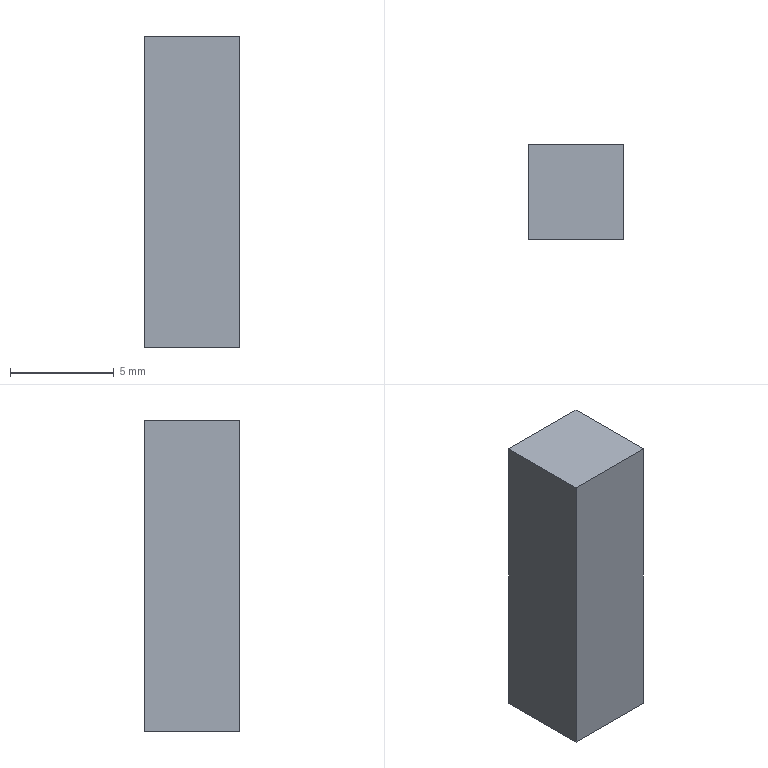Part | STEP file | Harpoon track spring pin | 1 solid | 6 faces | box 4.58 x 4.58 x 15 mm | volume 314.646 mm3 | plane 6
STEP:
#1=CARTESIAN_POINT('',(0.,0.,0.));
#2=DIRECTION('',(0.,0.,1.));
#3=DIRECTION('',(1.,0.,0.));
#4=AXIS2_PLACEMENT_3D('',#1,#2,#3);
#5=CARTESIAN_POINT('',(0.,4.58,0.));
#6=VERTEX_POINT('',#5);
#7=CARTESIAN_POINT('',(0.,0.,0.));
#8=VERTEX_POINT('',#7);
#9=CARTESIAN_POINT('',(0.,0.,0.));
#10=DIRECTION('',(0.,-1.,0.));
#11=VECTOR('',#10,1.);
#12=LINE('',#9,#11);
#13=CARTESIAN_POINT('',(0.,0.,15.));
#14=DIRECTION('',(1.,0.,0.));
#15=DIRECTION('',(0.,1.,0.));
#16=AXIS2_PLACEMENT_3D('',#13,#14,#15);
#17=PLANE('',#16);
#18=CARTESIAN_POINT('',(0.,-15.));
#19=DIRECTION('',(-1.,0.));
#20=VECTOR('',#19,1.);
#21=LINE('',#18,#20);
#22=(GEOMETRIC_REPRESENTATION_CONTEXT(2)PARAMETRIC_REPRESENTATION_CONTEXT()REPRESENTATION_CONTEXT('',''));
#23=DEFINITIONAL_REPRESENTATION('',(#21),#22);
#24=PCURVE('',#17,#23);
#25=CARTESIAN_POINT('',(0.,4.58,0.));
#26=DIRECTION('',(0.,0.,-1.));
#27=DIRECTION('',(-1.,0.,0.));
#28=AXIS2_PLACEMENT_3D('',#25,#26,#27);
#29=PLANE('',#28);
#30=CARTESIAN_POINT('',(0.,-4.58));
#31=DIRECTION('',(0.,-1.));
#32=VECTOR('',#31,1.);
#33=LINE('',#30,#32);
#34=(GEOMETRIC_REPRESENTATION_CONTEXT(2)PARAMETRIC_REPRESENTATION_CONTEXT()REPRESENTATION_CONTEXT('',''));
#35=DEFINITIONAL_REPRESENTATION('',(#33),#34);
#36=PCURVE('',#29,#35);
#37=SURFACE_CURVE('',#12,(#24,#36),.PCURVE_S1.);
#38=EDGE_CURVE('',#6,#8,#37,.T.);
#39=ORIENTED_EDGE('',*,*,#38,.T.);
#40=CARTESIAN_POINT('',(0.,0.,15.));
#41=VERTEX_POINT('',#40);
#42=CARTESIAN_POINT('',(0.,0.,15.));
#43=DIRECTION('',(0.,0.,-1.));
#44=VECTOR('',#43,1.);
#45=LINE('',#42,#44);
#46=CARTESIAN_POINT('',(0.,0.));
#47=DIRECTION('',(0.,-1.));
#48=VECTOR('',#47,1.);
#49=LINE('',#46,#48);
#50=(GEOMETRIC_REPRESENTATION_CONTEXT(2)PARAMETRIC_REPRESENTATION_CONTEXT()REPRESENTATION_CONTEXT('',''));
#51=DEFINITIONAL_REPRESENTATION('',(#49),#50);
#52=PCURVE('',#17,#51);
#53=CARTESIAN_POINT('',(0.,0.,15.));
#54=DIRECTION('',(0.,1.,0.));
#55=DIRECTION('',(0.,0.,1.));
#56=AXIS2_PLACEMENT_3D('',#53,#54,#55);
#57=PLANE('',#56);
#58=CARTESIAN_POINT('',(0.,0.));
#59=DIRECTION('',(-1.,0.));
#60=VECTOR('',#59,1.);
#61=LINE('',#58,#60);
#62=(GEOMETRIC_REPRESENTATION_CONTEXT(2)PARAMETRIC_REPRESENTATION_CONTEXT()REPRESENTATION_CONTEXT('',''));
#63=DEFINITIONAL_REPRESENTATION('',(#61),#62);
#64=PCURVE('',#57,#63);
#65=SURFACE_CURVE('',#45,(#52,#64),.PCURVE_S1.);
#66=EDGE_CURVE('',#41,#8,#65,.T.);
#67=ORIENTED_EDGE('',*,*,#66,.F.);
#68=CARTESIAN_POINT('',(0.,4.58,15.));
#69=VERTEX_POINT('',#68);
#70=CARTESIAN_POINT('',(0.,0.,15.));
#71=DIRECTION('',(0.,-1.,0.));
#72=VECTOR('',#71,1.);
#73=LINE('',#70,#72);
#74=CARTESIAN_POINT('',(0.,0.));
#75=DIRECTION('',(-1.,0.));
#76=VECTOR('',#75,1.);
#77=LINE('',#74,#76);
#78=(GEOMETRIC_REPRESENTATION_CONTEXT(2)PARAMETRIC_REPRESENTATION_CONTEXT()REPRESENTATION_CONTEXT('',''));
#79=DEFINITIONAL_REPRESENTATION('',(#77),#78);
#80=PCURVE('',#17,#79);
#81=CARTESIAN_POINT('',(0.,4.58,15.));
#82=DIRECTION('',(0.,0.,-1.));
#83=DIRECTION('',(-1.,0.,0.));
#84=AXIS2_PLACEMENT_3D('',#81,#82,#83);
#85=PLANE('',#84);
#86=CARTESIAN_POINT('',(0.,-4.58));
#87=DIRECTION('',(0.,-1.));
#88=VECTOR('',#87,1.);
#89=LINE('',#86,#88);
#90=(GEOMETRIC_REPRESENTATION_CONTEXT(2)PARAMETRIC_REPRESENTATION_CONTEXT()REPRESENTATION_CONTEXT('',''));
#91=DEFINITIONAL_REPRESENTATION('',(#89),#90);
#92=PCURVE('',#85,#91);
#93=SURFACE_CURVE('',#73,(#80,#92),.PCURVE_S1.);
#94=EDGE_CURVE('',#69,#41,#93,.T.);
#95=ORIENTED_EDGE('',*,*,#94,.F.);
#96=CARTESIAN_POINT('',(0.,4.58,15.));
#97=DIRECTION('',(0.,0.,-1.));
#98=VECTOR('',#97,1.);
#99=LINE('',#96,#98);
#100=CARTESIAN_POINT('',(4.58,0.));
#101=DIRECTION('',(0.,-1.));
#102=VECTOR('',#101,1.);
#103=LINE('',#100,#102);
#104=(GEOMETRIC_REPRESENTATION_CONTEXT(2)PARAMETRIC_REPRESENTATION_CONTEXT()REPRESENTATION_CONTEXT('',''));
#105=DEFINITIONAL_REPRESENTATION('',(#103),#104);
#106=PCURVE('',#17,#105);
#107=CARTESIAN_POINT('',(0.,4.58,15.));
#108=DIRECTION('',(0.,-1.,0.));
#109=DIRECTION('',(0.,0.,-1.));
#110=AXIS2_PLACEMENT_3D('',#107,#108,#109);
#111=PLANE('',#110);
#112=CARTESIAN_POINT('',(0.,0.));
#113=DIRECTION('',(1.,0.));
#114=VECTOR('',#113,1.);
#115=LINE('',#112,#114);
#116=(GEOMETRIC_REPRESENTATION_CONTEXT(2)PARAMETRIC_REPRESENTATION_CONTEXT()REPRESENTATION_CONTEXT('',''));
#117=DEFINITIONAL_REPRESENTATION('',(#115),#116);
#118=PCURVE('',#111,#117);
#119=SURFACE_CURVE('',#99,(#106,#118),.PCURVE_S1.);
#120=EDGE_CURVE('',#69,#6,#119,.T.);
#121=ORIENTED_EDGE('',*,*,#120,.T.);
#122=EDGE_LOOP('',(#39,#67,#95,#121));
#123=FACE_BOUND('',#122,.T.);
#124=ADVANCED_FACE('',(#123),#17,.F.);
#125=CARTESIAN_POINT('',(4.58,0.,0.));
#126=VERTEX_POINT('',#125);
#127=CARTESIAN_POINT('',(0.,0.,0.));
#128=DIRECTION('',(1.,0.,0.));
#129=VECTOR('',#128,1.);
#130=LINE('',#127,#129);
#131=CARTESIAN_POINT('',(-15.,0.));
#132=DIRECTION('',(0.,1.));
#133=VECTOR('',#132,1.);
#134=LINE('',#131,#133);
#135=(GEOMETRIC_REPRESENTATION_CONTEXT(2)PARAMETRIC_REPRESENTATION_CONTEXT()REPRESENTATION_CONTEXT('',''));
#136=DEFINITIONAL_REPRESENTATION('',(#134),#135);
#137=PCURVE('',#57,#136);
#138=CARTESIAN_POINT('',(0.,-4.58));
#139=DIRECTION('',(-1.,0.));
#140=VECTOR('',#139,1.);
#141=LINE('',#138,#140);
#142=(GEOMETRIC_REPRESENTATION_CONTEXT(2)PARAMETRIC_REPRESENTATION_CONTEXT()REPRESENTATION_CONTEXT('',''));
#143=DEFINITIONAL_REPRESENTATION('',(#141),#142);
#144=PCURVE('',#29,#143);
#145=SURFACE_CURVE('',#130,(#137,#144),.PCURVE_S1.);
#146=EDGE_CURVE('',#8,#126,#145,.T.);
#147=ORIENTED_EDGE('',*,*,#146,.T.);
#148=CARTESIAN_POINT('',(4.58,0.,15.));
#149=VERTEX_POINT('',#148);
#150=CARTESIAN_POINT('',(4.58,0.,15.));
#151=DIRECTION('',(0.,0.,-1.));
#152=VECTOR('',#151,1.);
#153=LINE('',#150,#152);
#154=CARTESIAN_POINT('',(0.,4.58));
#155=DIRECTION('',(-1.,0.));
#156=VECTOR('',#155,1.);
#157=LINE('',#154,#156);
#158=(GEOMETRIC_REPRESENTATION_CONTEXT(2)PARAMETRIC_REPRESENTATION_CONTEXT()REPRESENTATION_CONTEXT('',''));
#159=DEFINITIONAL_REPRESENTATION('',(#157),#158);
#160=PCURVE('',#57,#159);
#161=CARTESIAN_POINT('',(4.58,0.,15.));
#162=DIRECTION('',(-1.,0.,0.));
#163=DIRECTION('',(0.,0.,1.));
#164=AXIS2_PLACEMENT_3D('',#161,#162,#163);
#165=PLANE('',#164);
#166=CARTESIAN_POINT('',(0.,0.));
#167=DIRECTION('',(-1.,0.));
#168=VECTOR('',#167,1.);
#169=LINE('',#166,#168);
#170=(GEOMETRIC_REPRESENTATION_CONTEXT(2)PARAMETRIC_REPRESENTATION_CONTEXT()REPRESENTATION_CONTEXT('',''));
#171=DEFINITIONAL_REPRESENTATION('',(#169),#170);
#172=PCURVE('',#165,#171);
#173=SURFACE_CURVE('',#153,(#160,#172),.PCURVE_S1.);
#174=EDGE_CURVE('',#149,#126,#173,.T.);
#175=ORIENTED_EDGE('',*,*,#174,.F.);
#176=CARTESIAN_POINT('',(0.,0.,15.));
#177=DIRECTION('',(1.,0.,0.));
#178=VECTOR('',#177,1.);
#179=LINE('',#176,#178);
#180=CARTESIAN_POINT('',(0.,0.));
#181=DIRECTION('',(0.,1.));
#182=VECTOR('',#181,1.);
#183=LINE('',#180,#182);
#184=(GEOMETRIC_REPRESENTATION_CONTEXT(2)PARAMETRIC_REPRESENTATION_CONTEXT()REPRESENTATION_CONTEXT('',''));
#185=DEFINITIONAL_REPRESENTATION('',(#183),#184);
#186=PCURVE('',#57,#185);
#187=CARTESIAN_POINT('',(0.,-4.58));
#188=DIRECTION('',(-1.,0.));
#189=VECTOR('',#188,1.);
#190=LINE('',#187,#189);
#191=(GEOMETRIC_REPRESENTATION_CONTEXT(2)PARAMETRIC_REPRESENTATION_CONTEXT()REPRESENTATION_CONTEXT('',''));
#192=DEFINITIONAL_REPRESENTATION('',(#190),#191);
#193=PCURVE('',#85,#192);
#194=SURFACE_CURVE('',#179,(#186,#193),.PCURVE_S1.);
#195=EDGE_CURVE('',#41,#149,#194,.T.);
#196=ORIENTED_EDGE('',*,*,#195,.F.);
#197=ORIENTED_EDGE('',*,*,#66,.T.);
#198=EDGE_LOOP('',(#147,#175,#196,#197));
#199=FACE_BOUND('',#198,.T.);
#200=ADVANCED_FACE('',(#199),#57,.F.);
#201=CARTESIAN_POINT('',(4.58,4.58,0.));
#202=VERTEX_POINT('',#201);
#203=CARTESIAN_POINT('',(4.58,0.,0.));
#204=DIRECTION('',(0.,1.,0.));
#205=VECTOR('',#204,1.);
#206=LINE('',#203,#205);
#207=CARTESIAN_POINT('',(-15.,0.));
#208=DIRECTION('',(0.,1.));
#209=VECTOR('',#208,1.);
#210=LINE('',#207,#209);
#211=(GEOMETRIC_REPRESENTATION_CONTEXT(2)PARAMETRIC_REPRESENTATION_CONTEXT()REPRESENTATION_CONTEXT('',''));
#212=DEFINITIONAL_REPRESENTATION('',(#210),#211);
#213=PCURVE('',#165,#212);
#214=CARTESIAN_POINT('',(-4.58,-4.58));
#215=DIRECTION('',(0.,1.));
#216=VECTOR('',#215,1.);
#217=LINE('',#214,#216);
#218=(GEOMETRIC_REPRESENTATION_CONTEXT(2)PARAMETRIC_REPRESENTATION_CONTEXT()REPRESENTATION_CONTEXT('',''));
#219=DEFINITIONAL_REPRESENTATION('',(#217),#218);
#220=PCURVE('',#29,#219);
#221=SURFACE_CURVE('',#206,(#213,#220),.PCURVE_S1.);
#222=EDGE_CURVE('',#126,#202,#221,.T.);
#223=ORIENTED_EDGE('',*,*,#222,.T.);
#224=CARTESIAN_POINT('',(4.58,4.58,15.));
#225=VERTEX_POINT('',#224);
#226=CARTESIAN_POINT('',(4.58,4.58,15.));
#227=DIRECTION('',(0.,0.,-1.));
#228=VECTOR('',#227,1.);
#229=LINE('',#226,#228);
#230=CARTESIAN_POINT('',(0.,4.58));
#231=DIRECTION('',(-1.,0.));
#232=VECTOR('',#231,1.);
#233=LINE('',#230,#232);
#234=(GEOMETRIC_REPRESENTATION_CONTEXT(2)PARAMETRIC_REPRESENTATION_CONTEXT()REPRESENTATION_CONTEXT('',''));
#235=DEFINITIONAL_REPRESENTATION('',(#233),#234);
#236=PCURVE('',#165,#235);
#237=CARTESIAN_POINT('',(0.,4.58));
#238=DIRECTION('',(1.,0.));
#239=VECTOR('',#238,1.);
#240=LINE('',#237,#239);
#241=(GEOMETRIC_REPRESENTATION_CONTEXT(2)PARAMETRIC_REPRESENTATION_CONTEXT()REPRESENTATION_CONTEXT('',''));
#242=DEFINITIONAL_REPRESENTATION('',(#240),#241);
#243=PCURVE('',#111,#242);
#244=SURFACE_CURVE('',#229,(#236,#243),.PCURVE_S1.);
#245=EDGE_CURVE('',#225,#202,#244,.T.);
#246=ORIENTED_EDGE('',*,*,#245,.F.);
#247=CARTESIAN_POINT('',(4.58,0.,15.));
#248=DIRECTION('',(0.,1.,0.));
#249=VECTOR('',#248,1.);
#250=LINE('',#247,#249);
#251=CARTESIAN_POINT('',(0.,0.));
#252=DIRECTION('',(0.,1.));
#253=VECTOR('',#252,1.);
#254=LINE('',#251,#253);
#255=(GEOMETRIC_REPRESENTATION_CONTEXT(2)PARAMETRIC_REPRESENTATION_CONTEXT()REPRESENTATION_CONTEXT('',''));
#256=DEFINITIONAL_REPRESENTATION('',(#254),#255);
#257=PCURVE('',#165,#256);
#258=CARTESIAN_POINT('',(-4.58,-4.58));
#259=DIRECTION('',(0.,1.));
#260=VECTOR('',#259,1.);
#261=LINE('',#258,#260);
#262=(GEOMETRIC_REPRESENTATION_CONTEXT(2)PARAMETRIC_REPRESENTATION_CONTEXT()REPRESENTATION_CONTEXT('',''));
#263=DEFINITIONAL_REPRESENTATION('',(#261),#262);
#264=PCURVE('',#85,#263);
#265=SURFACE_CURVE('',#250,(#257,#264),.PCURVE_S1.);
#266=EDGE_CURVE('',#149,#225,#265,.T.);
#267=ORIENTED_EDGE('',*,*,#266,.F.);
#268=ORIENTED_EDGE('',*,*,#174,.T.);
#269=EDGE_LOOP('',(#223,#246,#267,#268));
#270=FACE_BOUND('',#269,.T.);
#271=ADVANCED_FACE('',(#270),#165,.F.);
#272=CARTESIAN_POINT('',(0.,4.58,0.));
#273=DIRECTION('',(-1.,0.,0.));
#274=VECTOR('',#273,1.);
#275=LINE('',#272,#274);
#276=CARTESIAN_POINT('',(15.,0.));
#277=DIRECTION('',(0.,-1.));
#278=VECTOR('',#277,1.);
#279=LINE('',#276,#278);
#280=(GEOMETRIC_REPRESENTATION_CONTEXT(2)PARAMETRIC_REPRESENTATION_CONTEXT()REPRESENTATION_CONTEXT('',''));
#281=DEFINITIONAL_REPRESENTATION('',(#279),#280);
#282=PCURVE('',#111,#281);
#283=CARTESIAN_POINT('',(0.,0.));
#284=DIRECTION('',(1.,0.));
#285=VECTOR('',#284,1.);
#286=LINE('',#283,#285);
#287=(GEOMETRIC_REPRESENTATION_CONTEXT(2)PARAMETRIC_REPRESENTATION_CONTEXT()REPRESENTATION_CONTEXT('',''));
#288=DEFINITIONAL_REPRESENTATION('',(#286),#287);
#289=PCURVE('',#29,#288);
#290=SURFACE_CURVE('',#275,(#282,#289),.PCURVE_S1.);
#291=EDGE_CURVE('',#202,#6,#290,.T.);
#292=ORIENTED_EDGE('',*,*,#291,.T.);
#293=ORIENTED_EDGE('',*,*,#120,.F.);
#294=CARTESIAN_POINT('',(0.,4.58,15.));
#295=DIRECTION('',(-1.,0.,0.));
#296=VECTOR('',#295,1.);
#297=LINE('',#294,#296);
#298=CARTESIAN_POINT('',(0.,0.));
#299=DIRECTION('',(0.,-1.));
#300=VECTOR('',#299,1.);
#301=LINE('',#298,#300);
#302=(GEOMETRIC_REPRESENTATION_CONTEXT(2)PARAMETRIC_REPRESENTATION_CONTEXT()REPRESENTATION_CONTEXT('',''));
#303=DEFINITIONAL_REPRESENTATION('',(#301),#302);
#304=PCURVE('',#111,#303);
#305=CARTESIAN_POINT('',(0.,0.));
#306=DIRECTION('',(1.,0.));
#307=VECTOR('',#306,1.);
#308=LINE('',#305,#307);
#309=(GEOMETRIC_REPRESENTATION_CONTEXT(2)PARAMETRIC_REPRESENTATION_CONTEXT()REPRESENTATION_CONTEXT('',''));
#310=DEFINITIONAL_REPRESENTATION('',(#308),#309);
#311=PCURVE('',#85,#310);
#312=SURFACE_CURVE('',#297,(#304,#311),.PCURVE_S1.);
#313=EDGE_CURVE('',#225,#69,#312,.T.);
#314=ORIENTED_EDGE('',*,*,#313,.F.);
#315=ORIENTED_EDGE('',*,*,#245,.T.);
#316=EDGE_LOOP('',(#292,#293,#314,#315));
#317=FACE_BOUND('',#316,.T.);
#318=ADVANCED_FACE('',(#317),#111,.F.);
#319=ORIENTED_EDGE('',*,*,#94,.T.);
#320=ORIENTED_EDGE('',*,*,#195,.T.);
#321=ORIENTED_EDGE('',*,*,#266,.T.);
#322=ORIENTED_EDGE('',*,*,#313,.T.);
#323=EDGE_LOOP('',(#319,#320,#321,#322));
#324=FACE_BOUND('',#323,.T.);
#325=ADVANCED_FACE('',(#324),#85,.F.);
#326=ORIENTED_EDGE('',*,*,#38,.F.);
#327=ORIENTED_EDGE('',*,*,#291,.F.);
#328=ORIENTED_EDGE('',*,*,#222,.F.);
#329=ORIENTED_EDGE('',*,*,#146,.F.);
#330=EDGE_LOOP('',(#326,#327,#328,#329));
#331=FACE_BOUND('',#330,.T.);
#332=ADVANCED_FACE('',(#331),#29,.T.);
#333=CLOSED_SHELL('',(#124,#200,#271,#318,#325,#332));
#334=MANIFOLD_SOLID_BREP('',#333);
#335=(LENGTH_UNIT()NAMED_UNIT(*)SI_UNIT(.MILLI.,.METRE.));
#336=UNCERTAINTY_MEASURE_WITH_UNIT(LENGTH_MEASURE(0.0000001),#335,'','');
#337=(NAMED_UNIT(*)PLANE_ANGLE_UNIT()SI_UNIT($,.RADIAN.));
#338=(NAMED_UNIT(*)SI_UNIT($,.STERADIAN.)SOLID_ANGLE_UNIT());
#339=(GEOMETRIC_REPRESENTATION_CONTEXT(3)GLOBAL_UNCERTAINTY_ASSIGNED_CONTEXT((#336))GLOBAL_UNIT_ASSIGNED_CONTEXT((#335,#337,#338))REPRESENTATION_CONTEXT('',''));
#340=ADVANCED_BREP_SHAPE_REPRESENTATION('',(#4,#334),#339);